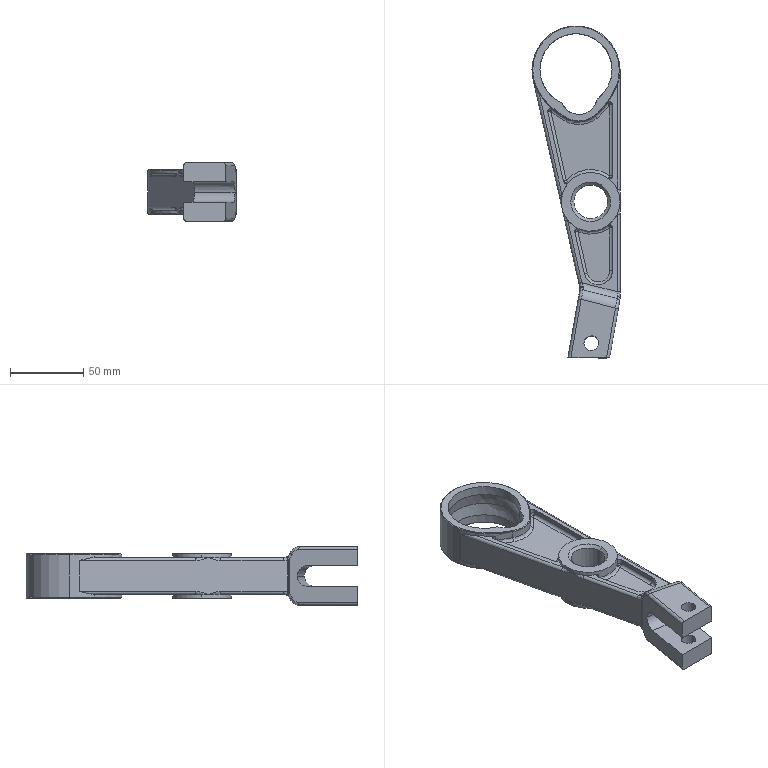Part | SolidWorks | features BaseBody 1 | 1 solid | 182 faces | box 60 x 226.322 x 40 mm | volume 155209 mm3 | cylinder 71 | spline 60 | plane 32 | cone 19 | commonest cylinder face diameters 4 x36 10 x6 49.143 x6 14 x4 40 x4 60 x4